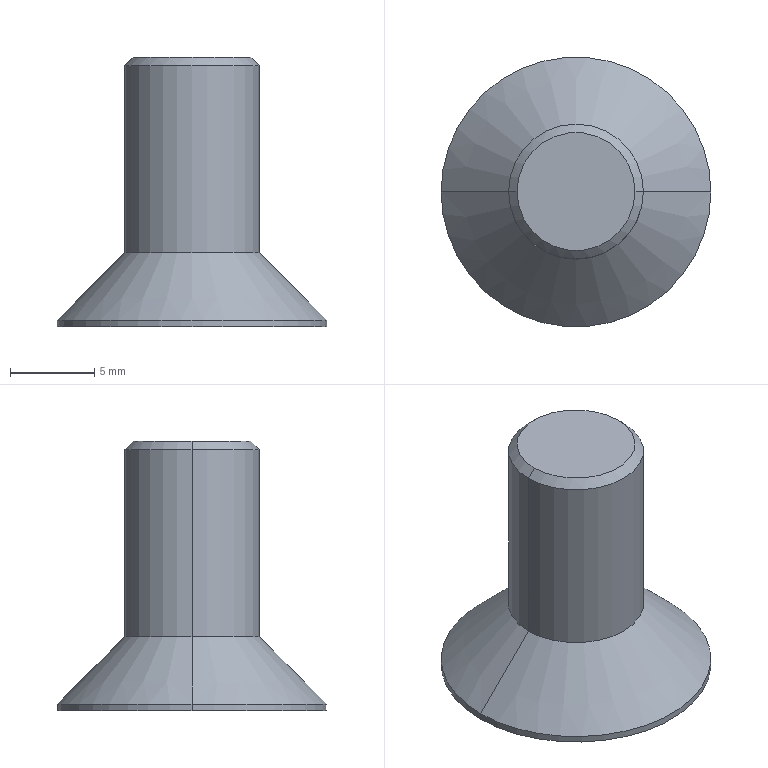Part | NX | features BREP 1 | 1 solid | 24 faces | box 16 x 16 x 16 mm | volume 988.606 mm3 | plane 14 | cone 6 | cylinder 4 | commonest cylinder face diameters 8 x2 16 x2
STEP:
#1=CARTESIAN_POINT('',(0.,0.,5.732));
#2=VERTEX_POINT('',#1);
#3=CARTESIAN_POINT('',(-3.,0.,4.));
#4=VERTEX_POINT('',#3);
#5=CARTESIAN_POINT('',(-3.,0.,4.));
#6=DIRECTION('',(-0.866,0.,-0.5));
#7=VECTOR('',#6,1000.);
#8=LINE('',#5,#7);
#9=EDGE_CURVE('',#2,#4,#8,.T.);
#10=ORIENTED_EDGE('',*,*,#9,.F.);
#11=CARTESIAN_POINT('',(3.,0.,4.));
#12=VERTEX_POINT('',#11);
#13=CARTESIAN_POINT('',(3.,0.,4.));
#14=DIRECTION('',(0.866,0.,-0.5));
#15=VECTOR('',#14,1000.);
#16=LINE('',#13,#15);
#17=EDGE_CURVE('',#2,#12,#16,.T.);
#18=ORIENTED_EDGE('',*,*,#17,.T.);
#19=CARTESIAN_POINT('',(2.598,-1.5,4.));
#20=VERTEX_POINT('',#19);
#21=CARTESIAN_POINT('',(0.,0.,4.));
#22=DIRECTION('',(0.,0.,-1.));
#23=DIRECTION('',(-1.,0.,0.));
#24=AXIS2_PLACEMENT_3D('',#21,#22,#23);
#25=CIRCLE('',#24,3.);
#26=EDGE_CURVE('',#12,#20,#25,.T.);
#27=ORIENTED_EDGE('',*,*,#26,.T.);
#28=CARTESIAN_POINT('',(0.,-3.,4.));
#29=VERTEX_POINT('',#28);
#30=CARTESIAN_POINT('',(0.,0.,4.));
#31=DIRECTION('',(0.,0.,-1.));
#32=DIRECTION('',(-1.,0.,0.));
#33=AXIS2_PLACEMENT_3D('',#30,#31,#32);
#34=CIRCLE('',#33,3.);
#35=EDGE_CURVE('',#20,#29,#34,.T.);
#36=ORIENTED_EDGE('',*,*,#35,.T.);
#37=CARTESIAN_POINT('',(-2.598,-1.5,4.));
#38=VERTEX_POINT('',#37);
#39=CARTESIAN_POINT('',(0.,0.,4.));
#40=DIRECTION('',(0.,0.,-1.));
#41=DIRECTION('',(-1.,0.,0.));
#42=AXIS2_PLACEMENT_3D('',#39,#40,#41);
#43=CIRCLE('',#42,3.);
#44=EDGE_CURVE('',#29,#38,#43,.T.);
#45=ORIENTED_EDGE('',*,*,#44,.T.);
#46=CARTESIAN_POINT('',(0.,0.,4.));
#47=DIRECTION('',(0.,0.,-1.));
#48=DIRECTION('',(-1.,0.,0.));
#49=AXIS2_PLACEMENT_3D('',#46,#47,#48);
#50=CIRCLE('',#49,3.);
#51=EDGE_CURVE('',#38,#4,#50,.T.);
#52=ORIENTED_EDGE('',*,*,#51,.T.);
#53=EDGE_LOOP('',(#10,#18,#27,#36,#45,#52));
#54=FACE_BOUND('',#53,.T.);
#55=CARTESIAN_POINT('',(0.,0.,4.));
#56=DIRECTION('',(0.,0.,-1.));
#57=DIRECTION('',(-1.,0.,0.));
#58=AXIS2_PLACEMENT_3D('',#55,#56,#57);
#59=CONICAL_SURFACE('',#58,3.,1.047);
#60=ADVANCED_FACE('',(#54),#59,.F.);
#61=CARTESIAN_POINT('',(3.5,0.,16.));
#62=VERTEX_POINT('',#61);
#63=CARTESIAN_POINT('',(-3.5,0.,16.));
#64=VERTEX_POINT('',#63);
#65=CARTESIAN_POINT('',(0.,0.,16.));
#66=DIRECTION('',(0.,0.,1.));
#67=DIRECTION('',(1.,0.,0.));
#68=AXIS2_PLACEMENT_3D('',#65,#66,#67);
#69=CIRCLE('',#68,3.5);
#70=EDGE_CURVE('',#62,#64,#69,.T.);
#71=ORIENTED_EDGE('',*,*,#70,.F.);
#72=CARTESIAN_POINT('',(4.,0.,15.5));
#73=VERTEX_POINT('',#72);
#74=CARTESIAN_POINT('',(3.5,0.,16.));
#75=DIRECTION('',(0.7071,0.,-0.7071));
#76=VECTOR('',#75,1000.);
#77=LINE('',#74,#76);
#78=EDGE_CURVE('',#62,#73,#77,.T.);
#79=ORIENTED_EDGE('',*,*,#78,.T.);
#80=CARTESIAN_POINT('',(-4.,0.,15.5));
#81=VERTEX_POINT('',#80);
#82=CARTESIAN_POINT('',(0.,0.,15.5));
#83=DIRECTION('',(0.,0.,-1.));
#84=DIRECTION('',(1.,0.,0.));
#85=AXIS2_PLACEMENT_3D('',#82,#83,#84);
#86=CIRCLE('',#85,4.);
#87=EDGE_CURVE('',#81,#73,#86,.T.);
#88=ORIENTED_EDGE('',*,*,#87,.F.);
#89=CARTESIAN_POINT('',(-3.5,0.,16.));
#90=DIRECTION('',(-0.7071,0.,-0.7071));
#91=VECTOR('',#90,1000.);
#92=LINE('',#89,#91);
#93=EDGE_CURVE('',#64,#81,#92,.T.);
#94=ORIENTED_EDGE('',*,*,#93,.F.);
#95=EDGE_LOOP('',(#71,#79,#88,#94));
#96=FACE_BOUND('',#95,.T.);
#97=CARTESIAN_POINT('',(0.,0.,16.));
#98=DIRECTION('',(0.,0.,-1.));
#99=DIRECTION('',(-1.,0.,0.));
#100=AXIS2_PLACEMENT_3D('',#97,#98,#99);
#101=CONICAL_SURFACE('',#100,3.5,0.7854);
#102=ADVANCED_FACE('',(#96),#101,.T.);
#103=ORIENTED_EDGE('',*,*,#87,.T.);
#104=CARTESIAN_POINT('',(4.,0.,4.4));
#105=VERTEX_POINT('',#104);
#106=CARTESIAN_POINT('',(4.,0.,16.));
#107=DIRECTION('',(0.,0.,-1.));
#108=VECTOR('',#107,1000.);
#109=LINE('',#106,#108);
#110=EDGE_CURVE('',#73,#105,#109,.T.);
#111=ORIENTED_EDGE('',*,*,#110,.T.);
#112=CARTESIAN_POINT('',(-4.,0.,4.4));
#113=VERTEX_POINT('',#112);
#114=CARTESIAN_POINT('',(0.,0.,4.4));
#115=DIRECTION('',(0.,0.,1.));
#116=DIRECTION('',(1.,0.,0.));
#117=AXIS2_PLACEMENT_3D('',#114,#115,#116);
#118=CIRCLE('',#117,4.);
#119=EDGE_CURVE('',#105,#113,#118,.T.);
#120=ORIENTED_EDGE('',*,*,#119,.T.);
#121=CARTESIAN_POINT('',(-4.,0.,16.));
#122=DIRECTION('',(0.,0.,-1.));
#123=VECTOR('',#122,1000.);
#124=LINE('',#121,#123);
#125=EDGE_CURVE('',#81,#113,#124,.T.);
#126=ORIENTED_EDGE('',*,*,#125,.F.);
#127=EDGE_LOOP('',(#103,#111,#120,#126));
#128=FACE_BOUND('',#127,.T.);
#129=CARTESIAN_POINT('',(0.,0.,16.));
#130=DIRECTION('',(0.,0.,-1.));
#131=DIRECTION('',(-1.,0.,0.));
#132=AXIS2_PLACEMENT_3D('',#129,#130,#131);
#133=CYLINDRICAL_SURFACE('',#132,4.);
#134=ADVANCED_FACE('',(#128),#133,.T.);
#135=ORIENTED_EDGE('',*,*,#119,.F.);
#136=CARTESIAN_POINT('',(8.,0.,0.4));
#137=VERTEX_POINT('',#136);
#138=CARTESIAN_POINT('',(4.,0.,4.4));
#139=DIRECTION('',(0.7071,0.,-0.7071));
#140=VECTOR('',#139,1000.);
#141=LINE('',#138,#140);
#142=EDGE_CURVE('',#105,#137,#141,.T.);
#143=ORIENTED_EDGE('',*,*,#142,.T.);
#144=CARTESIAN_POINT('',(-8.,0.,0.4));
#145=VERTEX_POINT('',#144);
#146=CARTESIAN_POINT('',(0.,0.,0.4));
#147=DIRECTION('',(0.,0.,-1.));
#148=DIRECTION('',(1.,0.,0.));
#149=AXIS2_PLACEMENT_3D('',#146,#147,#148);
#150=CIRCLE('',#149,8.);
#151=EDGE_CURVE('',#145,#137,#150,.T.);
#152=ORIENTED_EDGE('',*,*,#151,.F.);
#153=CARTESIAN_POINT('',(-4.,0.,4.4));
#154=DIRECTION('',(-0.7071,0.,-0.7071));
#155=VECTOR('',#154,1000.);
#156=LINE('',#153,#155);
#157=EDGE_CURVE('',#113,#145,#156,.T.);
#158=ORIENTED_EDGE('',*,*,#157,.F.);
#159=EDGE_LOOP('',(#135,#143,#152,#158));
#160=FACE_BOUND('',#159,.T.);
#161=CARTESIAN_POINT('',(0.,0.,4.4));
#162=DIRECTION('',(0.,0.,-1.));
#163=DIRECTION('',(-1.,0.,0.));
#164=AXIS2_PLACEMENT_3D('',#161,#162,#163);
#165=CONICAL_SURFACE('',#164,4.,0.7854);
#166=ADVANCED_FACE('',(#160),#165,.T.);
#167=ORIENTED_EDGE('',*,*,#151,.T.);
#168=CARTESIAN_POINT('',(8.,0.,0.));
#169=VERTEX_POINT('',#168);
#170=CARTESIAN_POINT('',(8.,0.,4.4));
#171=DIRECTION('',(0.,0.,-1.));
#172=VECTOR('',#171,1000.);
#173=LINE('',#170,#172);
#174=EDGE_CURVE('',#137,#169,#173,.T.);
#175=ORIENTED_EDGE('',*,*,#174,.T.);
#176=CARTESIAN_POINT('',(-8.,0.,0.));
#177=VERTEX_POINT('',#176);
#178=CARTESIAN_POINT('',(0.,0.,0.));
#179=DIRECTION('',(0.,0.,1.));
#180=DIRECTION('',(1.,0.,0.));
#181=AXIS2_PLACEMENT_3D('',#178,#179,#180);
#182=CIRCLE('',#181,8.);
#183=EDGE_CURVE('',#169,#177,#182,.T.);
#184=ORIENTED_EDGE('',*,*,#183,.T.);
#185=CARTESIAN_POINT('',(-8.,0.,4.4));
#186=DIRECTION('',(0.,0.,-1.));
#187=VECTOR('',#186,1000.);
#188=LINE('',#185,#187);
#189=EDGE_CURVE('',#145,#177,#188,.T.);
#190=ORIENTED_EDGE('',*,*,#189,.F.);
#191=EDGE_LOOP('',(#167,#175,#184,#190));
#192=FACE_BOUND('',#191,.T.);
#193=CARTESIAN_POINT('',(0.,0.,4.4));
#194=DIRECTION('',(0.,0.,-1.));
#195=DIRECTION('',(-1.,0.,0.));
#196=AXIS2_PLACEMENT_3D('',#193,#194,#195);
#197=CYLINDRICAL_SURFACE('',#196,8.);
#198=ADVANCED_FACE('',(#192),#197,.T.);
#199=CARTESIAN_POINT('',(-2.598,1.5,4.));
#200=VERTEX_POINT('',#199);
#201=CARTESIAN_POINT('',(0.,3.,4.));
#202=VERTEX_POINT('',#201);
#203=CARTESIAN_POINT('',(0.,0.,4.));
#204=DIRECTION('',(0.,0.,-1.));
#205=DIRECTION('',(-1.,0.,0.));
#206=AXIS2_PLACEMENT_3D('',#203,#204,#205);
#207=CIRCLE('',#206,3.);
#208=EDGE_CURVE('',#200,#202,#207,.T.);
#209=ORIENTED_EDGE('',*,*,#208,.F.);
#210=CARTESIAN_POINT('',(-1.732,3.,4.));
#211=VERTEX_POINT('',#210);
#212=CARTESIAN_POINT('',(-3.464,0.,4.));
#213=DIRECTION('',(0.5,0.866,0.));
#214=VECTOR('',#213,1000.);
#215=LINE('',#212,#214);
#216=EDGE_CURVE('',#200,#211,#215,.T.);
#217=ORIENTED_EDGE('',*,*,#216,.T.);
#218=CARTESIAN_POINT('',(-1.732,3.,4.));
#219=DIRECTION('',(1.,0.,0.));
#220=VECTOR('',#219,1000.);
#221=LINE('',#218,#220);
#222=EDGE_CURVE('',#211,#202,#221,.T.);
#223=ORIENTED_EDGE('',*,*,#222,.T.);
#224=EDGE_LOOP('',(#209,#217,#223));
#225=FACE_BOUND('',#224,.T.);
#226=CARTESIAN_POINT('',(0.,0.,4.));
#227=DIRECTION('',(0.,0.,-1.));
#228=DIRECTION('',(0.,-1.,0.));
#229=AXIS2_PLACEMENT_3D('',#226,#227,#228);
#230=PLANE('',#229);
#231=ADVANCED_FACE('',(#225),#230,.T.);
#232=CARTESIAN_POINT('',(2.598,1.5,4.));
#233=VERTEX_POINT('',#232);
#234=CARTESIAN_POINT('',(0.,0.,4.));
#235=DIRECTION('',(0.,0.,-1.));
#236=DIRECTION('',(-1.,0.,0.));
#237=AXIS2_PLACEMENT_3D('',#234,#235,#236);
#238=CIRCLE('',#237,3.);
#239=EDGE_CURVE('',#202,#233,#238,.T.);
#240=ORIENTED_EDGE('',*,*,#239,.F.);
#241=CARTESIAN_POINT('',(1.732,3.,4.));
#242=VERTEX_POINT('',#241);
#243=CARTESIAN_POINT('',(-1.732,3.,4.));
#244=DIRECTION('',(1.,0.,0.));
#245=VECTOR('',#244,1000.);
#246=LINE('',#243,#245);
#247=EDGE_CURVE('',#202,#242,#246,.T.);
#248=ORIENTED_EDGE('',*,*,#247,.T.);
#249=CARTESIAN_POINT('',(1.732,3.,4.));
#250=DIRECTION('',(0.5,-0.866,0.));
#251=VECTOR('',#250,1000.);
#252=LINE('',#249,#251);
#253=EDGE_CURVE('',#242,#233,#252,.T.);
#254=ORIENTED_EDGE('',*,*,#253,.T.);
#255=EDGE_LOOP('',(#240,#248,#254));
#256=FACE_BOUND('',#255,.T.);
#257=CARTESIAN_POINT('',(0.,0.,4.));
#258=DIRECTION('',(0.,0.,-1.));
#259=DIRECTION('',(0.,-1.,0.));
#260=AXIS2_PLACEMENT_3D('',#257,#258,#259);
#261=PLANE('',#260);
#262=ADVANCED_FACE('',(#256),#261,.T.);
#263=CARTESIAN_POINT('',(0.,0.,4.));
#264=DIRECTION('',(0.,0.,-1.));
#265=DIRECTION('',(-1.,0.,0.));
#266=AXIS2_PLACEMENT_3D('',#263,#264,#265);
#267=CIRCLE('',#266,3.);
#268=EDGE_CURVE('',#233,#12,#267,.T.);
#269=ORIENTED_EDGE('',*,*,#268,.F.);
#270=CARTESIAN_POINT('',(3.464,0.,4.));
#271=VERTEX_POINT('',#270);
#272=CARTESIAN_POINT('',(1.732,3.,4.));
#273=DIRECTION('',(0.5,-0.866,0.));
#274=VECTOR('',#273,1000.);
#275=LINE('',#272,#274);
#276=EDGE_CURVE('',#233,#271,#275,.T.);
#277=ORIENTED_EDGE('',*,*,#276,.T.);
#278=CARTESIAN_POINT('',(3.464,0.,4.));
#279=DIRECTION('',(-0.5,-0.866,0.));
#280=VECTOR('',#279,1000.);
#281=LINE('',#278,#280);
#282=EDGE_CURVE('',#271,#20,#281,.T.);
#283=ORIENTED_EDGE('',*,*,#282,.T.);
#284=ORIENTED_EDGE('',*,*,#26,.F.);
#285=EDGE_LOOP('',(#269,#277,#283,#284));
#286=FACE_BOUND('',#285,.T.);
#287=CARTESIAN_POINT('',(0.,0.,4.));
#288=DIRECTION('',(0.,0.,-1.));
#289=DIRECTION('',(0.,-1.,0.));
#290=AXIS2_PLACEMENT_3D('',#287,#288,#289);
#291=PLANE('',#290);
#292=ADVANCED_FACE('',(#286),#291,.T.);
#293=ORIENTED_EDGE('',*,*,#35,.F.);
#294=CARTESIAN_POINT('',(1.732,-3.,4.));
#295=VERTEX_POINT('',#294);
#296=CARTESIAN_POINT('',(3.464,0.,4.));
#297=DIRECTION('',(-0.5,-0.866,0.));
#298=VECTOR('',#297,1000.);
#299=LINE('',#296,#298);
#300=EDGE_CURVE('',#20,#295,#299,.T.);
#301=ORIENTED_EDGE('',*,*,#300,.T.);
#302=CARTESIAN_POINT('',(1.732,-3.,4.));
#303=DIRECTION('',(-1.,0.,0.));
#304=VECTOR('',#303,1000.);
#305=LINE('',#302,#304);
#306=EDGE_CURVE('',#295,#29,#305,.T.);
#307=ORIENTED_EDGE('',*,*,#306,.T.);
#308=EDGE_LOOP('',(#293,#301,#307));
#309=FACE_BOUND('',#308,.T.);
#310=CARTESIAN_POINT('',(0.,0.,4.));
#311=DIRECTION('',(0.,0.,-1.));
#312=DIRECTION('',(0.,-1.,0.));
#313=AXIS2_PLACEMENT_3D('',#310,#311,#312);
#314=PLANE('',#313);
#315=ADVANCED_FACE('',(#309),#314,.T.);
#316=ORIENTED_EDGE('',*,*,#44,.F.);
#317=CARTESIAN_POINT('',(-1.732,-3.,4.));
#318=VERTEX_POINT('',#317);
#319=CARTESIAN_POINT('',(1.732,-3.,4.));
#320=DIRECTION('',(-1.,0.,0.));
#321=VECTOR('',#320,1000.);
#322=LINE('',#319,#321);
#323=EDGE_CURVE('',#29,#318,#322,.T.);
#324=ORIENTED_EDGE('',*,*,#323,.T.);
#325=CARTESIAN_POINT('',(-1.732,-3.,4.));
#326=DIRECTION('',(-0.5,0.866,0.));
#327=VECTOR('',#326,1000.);
#328=LINE('',#325,#327);
#329=EDGE_CURVE('',#318,#38,#328,.T.);
#330=ORIENTED_EDGE('',*,*,#329,.T.);
#331=EDGE_LOOP('',(#316,#324,#330));
#332=FACE_BOUND('',#331,.T.);
#333=CARTESIAN_POINT('',(0.,0.,4.));
#334=DIRECTION('',(0.,0.,-1.));
#335=DIRECTION('',(0.,-1.,0.));
#336=AXIS2_PLACEMENT_3D('',#333,#334,#335);
#337=PLANE('',#336);
#338=ADVANCED_FACE('',(#332),#337,.T.);
#339=ORIENTED_EDGE('',*,*,#174,.F.);
#340=CARTESIAN_POINT('',(0.,0.,0.4));
#341=DIRECTION('',(0.,0.,-1.));
#342=DIRECTION('',(1.,0.,0.));
#343=AXIS2_PLACEMENT_3D('',#340,#341,#342);
#344=CIRCLE('',#343,8.);
#345=EDGE_CURVE('',#137,#145,#344,.T.);
#346=ORIENTED_EDGE('',*,*,#345,.T.);
#347=ORIENTED_EDGE('',*,*,#189,.T.);
#348=CARTESIAN_POINT('',(0.,0.,0.));
#349=DIRECTION('',(0.,0.,1.));
#350=DIRECTION('',(1.,0.,0.));
#351=AXIS2_PLACEMENT_3D('',#348,#349,#350);
#352=CIRCLE('',#351,8.);
#353=EDGE_CURVE('',#177,#169,#352,.T.);
#354=ORIENTED_EDGE('',*,*,#353,.T.);
#355=EDGE_LOOP('',(#339,#346,#347,#354));
#356=FACE_BOUND('',#355,.T.);
#357=CARTESIAN_POINT('',(0.,0.,4.4));
#358=DIRECTION('',(0.,0.,-1.));
#359=DIRECTION('',(-1.,0.,0.));
#360=AXIS2_PLACEMENT_3D('',#357,#358,#359);
#361=CYLINDRICAL_SURFACE('',#360,8.);
#362=ADVANCED_FACE('',(#356),#361,.T.);
#363=ORIENTED_EDGE('',*,*,#353,.F.);
#364=ORIENTED_EDGE('',*,*,#183,.F.);
#365=EDGE_LOOP('',(#363,#364));
#366=FACE_BOUND('',#365,.T.);
#367=CARTESIAN_POINT('',(-1.732,3.,0.));
#368=VERTEX_POINT('',#367);
#369=CARTESIAN_POINT('',(1.732,3.,0.));
#370=VERTEX_POINT('',#369);
#371=CARTESIAN_POINT('',(-1.732,3.,0.));
#372=DIRECTION('',(1.,0.,0.));
#373=VECTOR('',#372,1000.);
#374=LINE('',#371,#373);
#375=EDGE_CURVE('',#368,#370,#374,.T.);
#376=ORIENTED_EDGE('',*,*,#375,.F.);
#377=CARTESIAN_POINT('',(-3.464,0.,0.));
#378=VERTEX_POINT('',#377);
#379=CARTESIAN_POINT('',(-3.464,0.,0.));
#380=DIRECTION('',(0.5,0.866,0.));
#381=VECTOR('',#380,1000.);
#382=LINE('',#379,#381);
#383=EDGE_CURVE('',#378,#368,#382,.T.);
#384=ORIENTED_EDGE('',*,*,#383,.F.);
#385=CARTESIAN_POINT('',(-1.732,-3.,0.));
#386=VERTEX_POINT('',#385);
#387=CARTESIAN_POINT('',(-1.732,-3.,0.));
#388=DIRECTION('',(-0.5,0.866,0.));
#389=VECTOR('',#388,1000.);
#390=LINE('',#387,#389);
#391=EDGE_CURVE('',#386,#378,#390,.T.);
#392=ORIENTED_EDGE('',*,*,#391,.F.);
#393=CARTESIAN_POINT('',(1.732,-3.,0.));
#394=VERTEX_POINT('',#393);
#395=CARTESIAN_POINT('',(1.732,-3.,0.));
#396=DIRECTION('',(-1.,0.,0.));
#397=VECTOR('',#396,1000.);
#398=LINE('',#395,#397);
#399=EDGE_CURVE('',#394,#386,#398,.T.);
#400=ORIENTED_EDGE('',*,*,#399,.F.);
#401=CARTESIAN_POINT('',(3.464,0.,0.));
#402=VERTEX_POINT('',#401);
#403=CARTESIAN_POINT('',(3.464,0.,0.));
#404=DIRECTION('',(-0.5,-0.866,0.));
#405=VECTOR('',#404,1000.);
#406=LINE('',#403,#405);
#407=EDGE_CURVE('',#402,#394,#406,.T.);
#408=ORIENTED_EDGE('',*,*,#407,.F.);
#409=CARTESIAN_POINT('',(1.732,3.,0.));
#410=DIRECTION('',(0.5,-0.866,0.));
#411=VECTOR('',#410,1000.);
#412=LINE('',#409,#411);
#413=EDGE_CURVE('',#370,#402,#412,.T.);
#414=ORIENTED_EDGE('',*,*,#413,.F.);
#415=EDGE_LOOP('',(#376,#384,#392,#400,#408,#414));
#416=FACE_BOUND('',#415,.T.);
#417=CARTESIAN_POINT('',(0.,0.,0.));
#418=DIRECTION('',(0.,0.,1.));
#419=DIRECTION('',(1.,0.,0.));
#420=AXIS2_PLACEMENT_3D('',#417,#418,#419);
#421=PLANE('',#420);
#422=ADVANCED_FACE('',(#366,#416),#421,.F.);
#423=ORIENTED_EDGE('',*,*,#142,.F.);
#424=CARTESIAN_POINT('',(0.,0.,4.4));
#425=DIRECTION('',(0.,0.,1.));
#426=DIRECTION('',(1.,0.,0.));
#427=AXIS2_PLACEMENT_3D('',#424,#425,#426);
#428=CIRCLE('',#427,4.);
#429=EDGE_CURVE('',#113,#105,#428,.T.);
#430=ORIENTED_EDGE('',*,*,#429,.F.);
#431=ORIENTED_EDGE('',*,*,#157,.T.);
#432=ORIENTED_EDGE('',*,*,#345,.F.);
#433=EDGE_LOOP('',(#423,#430,#431,#432));
#434=FACE_BOUND('',#433,.T.);
#435=CARTESIAN_POINT('',(0.,0.,4.4));
#436=DIRECTION('',(0.,0.,-1.));
#437=DIRECTION('',(-1.,0.,0.));
#438=AXIS2_PLACEMENT_3D('',#435,#436,#437);
#439=CONICAL_SURFACE('',#438,4.,0.7854);
#440=ADVANCED_FACE('',(#434),#439,.T.);
#441=ORIENTED_EDGE('',*,*,#110,.F.);
#442=CARTESIAN_POINT('',(0.,0.,15.5));
#443=DIRECTION('',(0.,0.,-1.));
#444=DIRECTION('',(1.,0.,0.));
#445=AXIS2_PLACEMENT_3D('',#442,#443,#444);
#446=CIRCLE('',#445,4.);
#447=EDGE_CURVE('',#73,#81,#446,.T.);
#448=ORIENTED_EDGE('',*,*,#447,.T.);
#449=ORIENTED_EDGE('',*,*,#125,.T.);
#450=ORIENTED_EDGE('',*,*,#429,.T.);
#451=EDGE_LOOP('',(#441,#448,#449,#450));
#452=FACE_BOUND('',#451,.T.);
#453=CARTESIAN_POINT('',(0.,0.,16.));
#454=DIRECTION('',(0.,0.,-1.));
#455=DIRECTION('',(-1.,0.,0.));
#456=AXIS2_PLACEMENT_3D('',#453,#454,#455);
#457=CYLINDRICAL_SURFACE('',#456,4.);
#458=ADVANCED_FACE('',(#452),#457,.T.);
#459=CARTESIAN_POINT('',(0.,0.,16.));
#460=DIRECTION('',(0.,0.,1.));
#461=DIRECTION('',(1.,0.,0.));
#462=AXIS2_PLACEMENT_3D('',#459,#460,#461);
#463=CIRCLE('',#462,3.5);
#464=EDGE_CURVE('',#64,#62,#463,.T.);
#465=ORIENTED_EDGE('',*,*,#464,.T.);
#466=ORIENTED_EDGE('',*,*,#70,.T.);
#467=EDGE_LOOP('',(#465,#466));
#468=FACE_BOUND('',#467,.T.);
#469=CARTESIAN_POINT('',(0.,0.,16.));
#470=DIRECTION('',(0.,0.,1.));
#471=DIRECTION('',(1.,0.,0.));
#472=AXIS2_PLACEMENT_3D('',#469,#470,#471);
#473=PLANE('',#472);
#474=ADVANCED_FACE('',(#468),#473,.T.);
#475=ORIENTED_EDGE('',*,*,#78,.F.);
#476=ORIENTED_EDGE('',*,*,#464,.F.);
#477=ORIENTED_EDGE('',*,*,#93,.T.);
#478=ORIENTED_EDGE('',*,*,#447,.F.);
#479=EDGE_LOOP('',(#475,#476,#477,#478));
#480=FACE_BOUND('',#479,.T.);
#481=CARTESIAN_POINT('',(0.,0.,16.));
#482=DIRECTION('',(0.,0.,-1.));
#483=DIRECTION('',(-1.,0.,0.));
#484=AXIS2_PLACEMENT_3D('',#481,#482,#483);
#485=CONICAL_SURFACE('',#484,3.5,0.7854);
#486=ADVANCED_FACE('',(#480),#485,.T.);
#487=ORIENTED_EDGE('',*,*,#383,.T.);
#488=CARTESIAN_POINT('',(-1.732,3.,4.));
#489=DIRECTION('',(0.,0.,-1.));
#490=VECTOR('',#489,1000.);
#491=LINE('',#488,#490);
#492=EDGE_CURVE('',#211,#368,#491,.T.);
#493=ORIENTED_EDGE('',*,*,#492,.F.);
#494=ORIENTED_EDGE('',*,*,#216,.F.);
#495=CARTESIAN_POINT('',(-3.464,0.,4.));
#496=VERTEX_POINT('',#495);
#497=CARTESIAN_POINT('',(-3.464,0.,4.));
#498=DIRECTION('',(0.5,0.866,0.));
#499=VECTOR('',#498,1000.);
#500=LINE('',#497,#499);
#501=EDGE_CURVE('',#496,#200,#500,.T.);
#502=ORIENTED_EDGE('',*,*,#501,.F.);
#503=CARTESIAN_POINT('',(-3.464,0.,4.));
#504=DIRECTION('',(0.,0.,-1.));
#505=VECTOR('',#504,1000.);
#506=LINE('',#503,#505);
#507=EDGE_CURVE('',#496,#378,#506,.T.);
#508=ORIENTED_EDGE('',*,*,#507,.T.);
#509=EDGE_LOOP('',(#487,#493,#494,#502,#508));
#510=FACE_BOUND('',#509,.T.);
#511=CARTESIAN_POINT('',(-3.464,0.,4.));
#512=DIRECTION('',(-0.866,0.5,0.));
#513=DIRECTION('',(0.,0.,1.));
#514=AXIS2_PLACEMENT_3D('',#511,#512,#513);
#515=PLANE('',#514);
#516=ADVANCED_FACE('',(#510),#515,.F.);
#517=ORIENTED_EDGE('',*,*,#391,.T.);
#518=ORIENTED_EDGE('',*,*,#507,.F.);
#519=CARTESIAN_POINT('',(-1.732,-3.,4.));
#520=DIRECTION('',(-0.5,0.866,0.));
#521=VECTOR('',#520,1000.);
#522=LINE('',#519,#521);
#523=EDGE_CURVE('',#38,#496,#522,.T.);
#524=ORIENTED_EDGE('',*,*,#523,.F.);
#525=ORIENTED_EDGE('',*,*,#329,.F.);
#526=CARTESIAN_POINT('',(-1.732,-3.,4.));
#527=DIRECTION('',(0.,0.,-1.));
#528=VECTOR('',#527,1000.);
#529=LINE('',#526,#528);
#530=EDGE_CURVE('',#318,#386,#529,.T.);
#531=ORIENTED_EDGE('',*,*,#530,.T.);
#532=EDGE_LOOP('',(#517,#518,#524,#525,#531));
#533=FACE_BOUND('',#532,.T.);
#534=CARTESIAN_POINT('',(-1.732,-3.,4.));
#535=DIRECTION('',(-0.866,-0.5,0.));
#536=DIRECTION('',(-0.5,0.866,0.));
#537=AXIS2_PLACEMENT_3D('',#534,#535,#536);
#538=PLANE('',#537);
#539=ADVANCED_FACE('',(#533),#538,.F.);
#540=ORIENTED_EDGE('',*,*,#399,.T.);
#541=ORIENTED_EDGE('',*,*,#530,.F.);
#542=ORIENTED_EDGE('',*,*,#323,.F.);
#543=ORIENTED_EDGE('',*,*,#306,.F.);
#544=CARTESIAN_POINT('',(1.732,-3.,4.));
#545=DIRECTION('',(0.,0.,-1.));
#546=VECTOR('',#545,1000.);
#547=LINE('',#544,#546);
#548=EDGE_CURVE('',#295,#394,#547,.T.);
#549=ORIENTED_EDGE('',*,*,#548,.T.);
#550=EDGE_LOOP('',(#540,#541,#542,#543,#549));
#551=FACE_BOUND('',#550,.T.);
#552=CARTESIAN_POINT('',(1.732,-3.,4.));
#553=DIRECTION('',(0.,-1.,0.));
#554=DIRECTION('',(0.,0.,-1.));
#555=AXIS2_PLACEMENT_3D('',#552,#553,#554);
#556=PLANE('',#555);
#557=ADVANCED_FACE('',(#551),#556,.F.);
#558=ORIENTED_EDGE('',*,*,#407,.T.);
#559=ORIENTED_EDGE('',*,*,#548,.F.);
#560=ORIENTED_EDGE('',*,*,#300,.F.);
#561=ORIENTED_EDGE('',*,*,#282,.F.);
#562=CARTESIAN_POINT('',(3.464,0.,4.));
#563=DIRECTION('',(0.,0.,-1.));
#564=VECTOR('',#563,1000.);
#565=LINE('',#562,#564);
#566=EDGE_CURVE('',#271,#402,#565,.T.);
#567=ORIENTED_EDGE('',*,*,#566,.T.);
#568=EDGE_LOOP('',(#558,#559,#560,#561,#567));
#569=FACE_BOUND('',#568,.T.);
#570=CARTESIAN_POINT('',(3.464,0.,4.));
#571=DIRECTION('',(0.866,-0.5,0.));
#572=DIRECTION('',(0.,0.,-1.));
#573=AXIS2_PLACEMENT_3D('',#570,#571,#572);
#574=PLANE('',#573);
#575=ADVANCED_FACE('',(#569),#574,.F.);
#576=ORIENTED_EDGE('',*,*,#413,.T.);
#577=ORIENTED_EDGE('',*,*,#566,.F.);
#578=ORIENTED_EDGE('',*,*,#276,.F.);
#579=ORIENTED_EDGE('',*,*,#253,.F.);
#580=CARTESIAN_POINT('',(1.732,3.,4.));
#581=DIRECTION('',(0.,0.,-1.));
#582=VECTOR('',#581,1000.);
#583=LINE('',#580,#582);
#584=EDGE_CURVE('',#242,#370,#583,.T.);
#585=ORIENTED_EDGE('',*,*,#584,.T.);
#586=EDGE_LOOP('',(#576,#577,#578,#579,#585));
#587=FACE_BOUND('',#586,.T.);
#588=CARTESIAN_POINT('',(1.732,3.,4.));
#589=DIRECTION('',(0.866,0.5,0.));
#590=DIRECTION('',(0.,0.,-1.));
#591=AXIS2_PLACEMENT_3D('',#588,#589,#590);
#592=PLANE('',#591);
#593=ADVANCED_FACE('',(#587),#592,.F.);
#594=ORIENTED_EDGE('',*,*,#375,.T.);
#595=ORIENTED_EDGE('',*,*,#584,.F.);
#596=ORIENTED_EDGE('',*,*,#247,.F.);
#597=ORIENTED_EDGE('',*,*,#222,.F.);
#598=ORIENTED_EDGE('',*,*,#492,.T.);
#599=EDGE_LOOP('',(#594,#595,#596,#597,#598));
#600=FACE_BOUND('',#599,.T.);
#601=CARTESIAN_POINT('',(-1.732,3.,4.));
#602=DIRECTION('',(0.,1.,0.));
#603=DIRECTION('',(1.,0.,0.));
#604=AXIS2_PLACEMENT_3D('',#601,#602,#603);
#605=PLANE('',#604);
#606=ADVANCED_FACE('',(#600),#605,.F.);
#607=ORIENTED_EDGE('',*,*,#51,.F.);
#608=ORIENTED_EDGE('',*,*,#523,.T.);
#609=ORIENTED_EDGE('',*,*,#501,.T.);
#610=CARTESIAN_POINT('',(0.,0.,4.));
#611=DIRECTION('',(0.,0.,-1.));
#612=DIRECTION('',(-1.,0.,0.));
#613=AXIS2_PLACEMENT_3D('',#610,#611,#612);
#614=CIRCLE('',#613,3.);
#615=EDGE_CURVE('',#4,#200,#614,.T.);
#616=ORIENTED_EDGE('',*,*,#615,.F.);
#617=EDGE_LOOP('',(#607,#608,#609,#616));
#618=FACE_BOUND('',#617,.T.);
#619=CARTESIAN_POINT('',(0.,0.,4.));
#620=DIRECTION('',(0.,0.,-1.));
#621=DIRECTION('',(0.,-1.,0.));
#622=AXIS2_PLACEMENT_3D('',#619,#620,#621);
#623=PLANE('',#622);
#624=ADVANCED_FACE('',(#618),#623,.T.);
#625=ORIENTED_EDGE('',*,*,#17,.F.);
#626=ORIENTED_EDGE('',*,*,#9,.T.);
#627=ORIENTED_EDGE('',*,*,#615,.T.);
#628=ORIENTED_EDGE('',*,*,#208,.T.);
#629=ORIENTED_EDGE('',*,*,#239,.T.);
#630=ORIENTED_EDGE('',*,*,#268,.T.);
#631=EDGE_LOOP('',(#625,#626,#627,#628,#629,#630));
#632=FACE_BOUND('',#631,.T.);
#633=CARTESIAN_POINT('',(0.,0.,4.));
#634=DIRECTION('',(0.,0.,-1.));
#635=DIRECTION('',(-1.,0.,0.));
#636=AXIS2_PLACEMENT_3D('',#633,#634,#635);
#637=CONICAL_SURFACE('',#636,3.,1.047);
#638=ADVANCED_FACE('',(#632),#637,.F.);
#639=CLOSED_SHELL('',(#60,#102,#134,#166,#198,#231,#262,#292,#315,#338,#362,#422,#440,#458,#474,#486,#516,#539,#557,#575,#593,#606,#624,#638));
#640=MANIFOLD_SOLID_BREP('',#639);
#641=(LENGTH_UNIT()NAMED_UNIT(*)SI_UNIT(.MILLI.,.METRE.));
#642=UNCERTAINTY_MEASURE_WITH_UNIT(LENGTH_MEASURE(0.00001),#641,'','');
#643=(NAMED_UNIT(*)PLANE_ANGLE_UNIT()SI_UNIT($,.RADIAN.));
#644=(NAMED_UNIT(*)SI_UNIT($,.STERADIAN.)SOLID_ANGLE_UNIT());
#645=(GEOMETRIC_REPRESENTATION_CONTEXT(3)GLOBAL_UNCERTAINTY_ASSIGNED_CONTEXT((#642))GLOBAL_UNIT_ASSIGNED_CONTEXT((#641,#643,#644))REPRESENTATION_CONTEXT('',''));
#646=ADVANCED_BREP_SHAPE_REPRESENTATION('',(#640),#645);